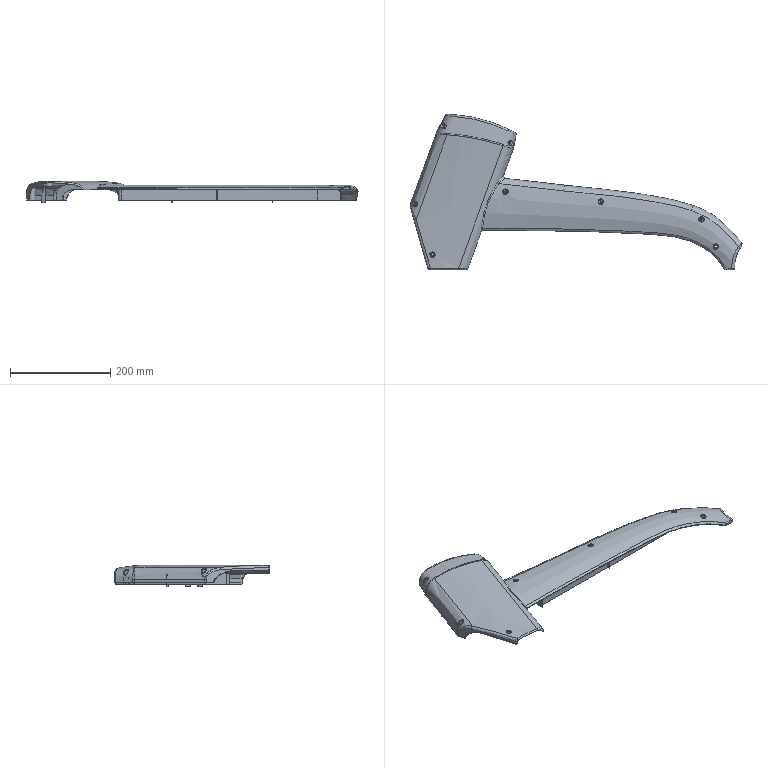Part | STEP file | PR12S0313~665.310.45LL | 1 solid | 289 faces | box 660.94 x 308.908 x 43 mm | volume 328028 mm3 | spline 119 | plane 94 | cylinder 65 | cone 7 | torus 4 | commonest cylinder face diameters 8.5 x11 12 x11 3.2 x6 2 x4 5 x4 9 x3